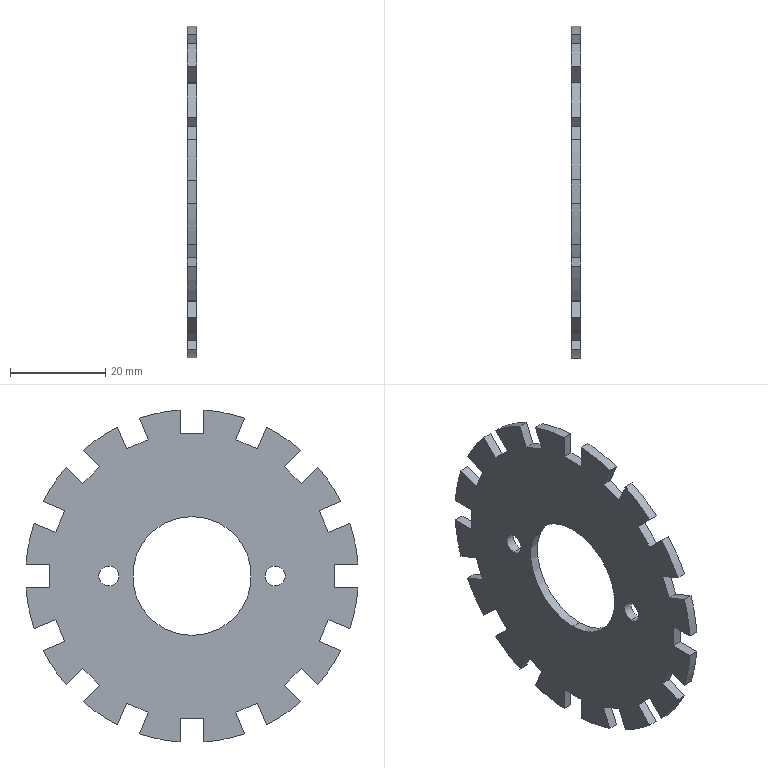Part | STEP file | 05-07 Alignment piece | 1 solid | 72 faces | box 2 x 69.821 x 69.821 mm | volume 5865 mm3 | plane 50 | cylinder 22 | commonest cylinder face diameters 70 x16 4.2 x4 25 x2